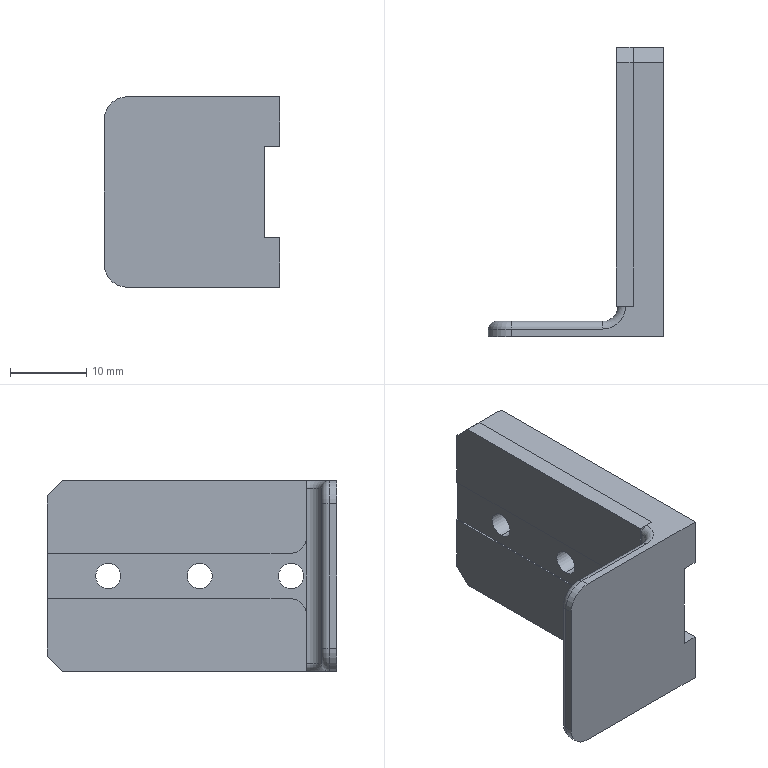Part | STEP file | 0-10-21 Cell support plate | 3 solids | 54 faces | box 23 x 38 x 25 mm | volume 5641 mm3 | plane 34 | cylinder 16 | torus 4 | commonest cylinder face diameters 3.3 x6 4 x5 2 x3 6 x2